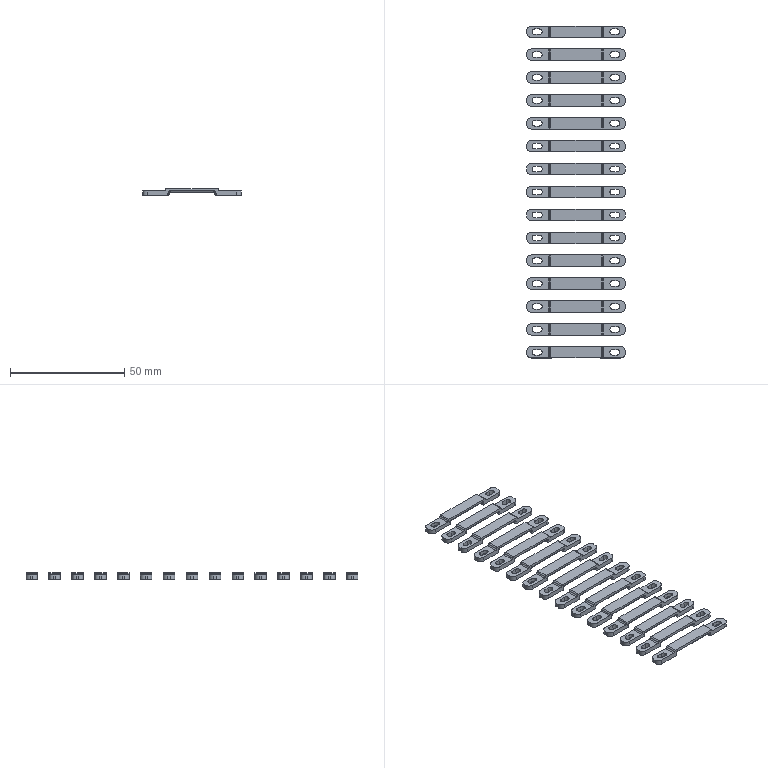NC program | NX | posted with a generic post | part box 43 x 145 x 3 mm
Lines 3017 to 4403 of 17881:
(PLANAR_MILL_COPY_COPY_COPY_COPY_COPY_COPY_1 , TOOL : D6A45)
N6014 T01 M6
N6016 G54
N6018 G17 G0 G90 X-73.9 Y-15.667 S9500 M3
N6020 G43 Z30. H1
N6022 Z0.5
N6024 G94 G1 Z-1. F1250.
N6026 G3 X-73.4 Y-14.801 R1.
N6028 G1 Y-10.5
N6030 X-73.383 Y-10.328
N6032 X-73.341 Y-10.108
N6034 G2 X-73.181 Y-9.746 R0.9
N6036 G1 X-73.065 Y-9.588
N6038 G2 X-72.775 Y-9.334 R0.9
N6040 G1 X-72.61 Y-9.243
N6042 G2 X-72.332 Y-9.145 R0.9
N6044 G1 X-72.156 Y-9.114
N6046 X-72. Y-9.1
N6048 X-68.
N6050 X-67.844 Y-9.114
N6052 X-67.668 Y-9.145
N6054 G2 X-67.39 Y-9.243 R0.9
N6056 G1 X-67.225 Y-9.334
N6058 G2 X-66.935 Y-9.588 R0.9
N6060 G1 X-66.819 Y-9.746
N6062 G2 X-66.659 Y-10.108 R0.9
N6064 G1 X-66.617 Y-10.328
N6066 X-66.6 Y-10.5
N6068 Y-19.5
N6070 G2 X-69.5 Y-22.4 R2.9
N6072 G1 X-70.5
N6074 G2 X-73.4 Y-19.5 R2.9
N6076 G1 Y-14.801
N6078 G3 X-73.9 Y-13.935 R1.
N6080 G1 Z0.5
N6082 G0 Z30.
N6084 X-70.2 Y-17.866
N6086 Z0.5
N6088 G1 Z-1.
N6090 G3 X-69.7 Y-17. R1.
N6092 G1 Y-16.
N6094 G3 X-70. Y-15.7 R0.3
N6096 X-70.3 Y-16. R0.3
N6098 G1 Y-18.
N6100 G3 X-70. Y-18.3 R0.3
N6102 X-69.7 Y-18. R0.3
N6104 G1 Y-17.
N6106 G3 X-70.2 Y-16.134 R1.
N6108 G1 Z0.5
N6110 G0 Z30.
N6112 X-60.2 Y-17.866
N6114 Z0.5
N6116 G1 Z-1.
N6118 G3 X-59.7 Y-17. R1.
N6120 G1 Y-16.
N6122 G3 X-60. Y-15.7 R0.3
N6124 X-60.3 Y-16. R0.3
N6126 G1 Y-18.
N6128 G3 X-60. Y-18.3 R0.3
N6130 X-59.7 Y-18. R0.3
N6132 G1 Y-17.
N6134 G3 X-60.2 Y-16.134 R1.
N6136 G1 Z0.5
N6138 G0 Z30.
N6140 X-56.1 Y-13.935
N6142 Z0.5
N6144 G1 Z-1.
N6146 G3 X-56.6 Y-14.801 R1.
N6148 G1 Y-19.5
N6150 G2 X-59.5 Y-22.4 R2.9
N6152 G1 X-60.5
N6154 G2 X-63.4 Y-19.5 R2.9
N6156 G1 Y-10.5
N6158 X-63.383 Y-10.328
N6160 X-63.341 Y-10.108
N6162 G2 X-63.181 Y-9.746 R0.9
N6164 G1 X-63.065 Y-9.588
N6166 G2 X-62.775 Y-9.334 R0.9
N6168 G1 X-62.61 Y-9.243
N6170 G2 X-62.332 Y-9.145 R0.9
N6172 G1 X-62.156 Y-9.114
N6174 X-62. Y-9.1
N6176 X-58.
N6178 X-57.844 Y-9.114
N6180 X-57.668 Y-9.145
N6182 G2 X-57.39 Y-9.243 R0.9
N6184 G1 X-57.225 Y-9.334
N6186 G2 X-56.935 Y-9.588 R0.9
N6188 G1 X-56.819 Y-9.746
N6190 G2 X-56.659 Y-10.108 R0.9
N6192 G1 X-56.617 Y-10.328
N6194 X-56.6 Y-10.5
N6196 Y-14.801
N6198 G3 X-56.1 Y-15.667 R1.
N6200 G1 Z0.5
N6202 G0 Z30.
N6204 X-53.9
N6206 Z0.5
N6208 G1 Z-1.
N6210 G3 X-53.4 Y-14.801 R1.
N6212 G1 Y-10.5
N6214 X-53.383 Y-10.328
N6216 X-53.341 Y-10.108
N6218 G2 X-53.181 Y-9.746 R0.9
N6220 G1 X-53.065 Y-9.588
N6222 G2 X-52.775 Y-9.334 R0.9
N6224 G1 X-52.61 Y-9.243
N6226 G2 X-52.332 Y-9.145 R0.9
N6228 G1 X-52.156 Y-9.114
N6230 X-52. Y-9.1
N6232 X-48.
N6234 X-47.844 Y-9.114
N6236 X-47.668 Y-9.145
N6238 G2 X-47.39 Y-9.243 R0.9
N6240 G1 X-47.225 Y-9.334
N6242 G2 X-46.935 Y-9.588 R0.9
N6244 G1 X-46.819 Y-9.746
N6246 G2 X-46.659 Y-10.108 R0.9
N6248 G1 X-46.617 Y-10.328
N6250 X-46.6 Y-10.5
N6252 Y-19.5
N6254 G2 X-49.5 Y-22.4 R2.9
N6256 G1 X-50.5
N6258 G2 X-53.4 Y-19.5 R2.9
N6260 G1 Y-14.801
N6262 G3 X-53.9 Y-13.935 R1.
N6264 G1 Z0.5
N6266 G0 Z30.
N6268 X-50.2 Y-17.866
N6270 Z0.5
N6272 G1 Z-1.
N6274 G3 X-49.7 Y-17. R1.
N6276 G1 Y-16.
N6278 G3 X-50. Y-15.7 R0.3
N6280 X-50.3 Y-16. R0.3
N6282 G1 Y-18.
N6284 G3 X-50. Y-18.3 R0.3
N6286 X-49.7 Y-18. R0.3
N6288 G1 Y-17.
N6290 G3 X-50.2 Y-16.134 R1.
N6292 G1 Z0.5
N6294 G0 Z30.
N6296 X-40.2 Y-17.866
N6298 Z0.5
N6300 G1 Z-1.
N6302 G3 X-39.7 Y-17. R1.
N6304 G1 Y-16.
N6306 G3 X-40. Y-15.7 R0.3
N6308 X-40.3 Y-16. R0.3
N6310 G1 Y-18.
N6312 G3 X-40. Y-18.3 R0.3
N6314 X-39.7 Y-18. R0.3
N6316 G1 Y-17.
N6318 G3 X-40.2 Y-16.134 R1.
N6320 G1 Z0.5
N6322 G0 Z30.
N6324 X-36.1 Y-13.935
N6326 Z0.5
N6328 G1 Z-1.
N6330 G3 X-36.6 Y-14.801 R1.
N6332 G1 Y-19.5
N6334 G2 X-39.5 Y-22.4 R2.9
N6336 G1 X-40.5
N6338 G2 X-43.4 Y-19.5 R2.9
N6340 G1 Y-10.5
N6342 X-43.383 Y-10.328
N6344 X-43.341 Y-10.108
N6346 G2 X-43.181 Y-9.746 R0.9
N6348 G1 X-43.065 Y-9.588
N6350 G2 X-42.775 Y-9.334 R0.9
N6352 G1 X-42.61 Y-9.243
N6354 G2 X-42.332 Y-9.145 R0.9
N6356 G1 X-42.156 Y-9.114
N6358 X-42. Y-9.1
N6360 X-38.
N6362 X-37.844 Y-9.114
N6364 X-37.668 Y-9.145
N6366 G2 X-37.39 Y-9.243 R0.9
N6368 G1 X-37.225 Y-9.334
N6370 G2 X-36.935 Y-9.588 R0.9
N6372 G1 X-36.819 Y-9.746
N6374 G2 X-36.659 Y-10.108 R0.9
N6376 G1 X-36.617 Y-10.328
N6378 X-36.6 Y-10.5
N6380 Y-14.801
N6382 G3 X-36.1 Y-15.667 R1.
N6384 G1 Z0.5
N6386 G0 Z30.
N6388 X-33.9
N6390 Z0.5
N6392 G1 Z-1.
N6394 G3 X-33.4 Y-14.801 R1.
N6396 G1 Y-10.5
N6398 X-33.383 Y-10.328
N6400 X-33.341 Y-10.108
N6402 G2 X-33.181 Y-9.746 R0.9
N6404 G1 X-33.065 Y-9.588
N6406 G2 X-32.775 Y-9.334 R0.9
N6408 G1 X-32.61 Y-9.243
N6410 G2 X-32.332 Y-9.145 R0.9
N6412 G1 X-32.156 Y-9.114
N6414 X-32. Y-9.1
N6416 X-28.
N6418 X-27.844 Y-9.114
N6420 X-27.668 Y-9.145
N6422 G2 X-27.39 Y-9.243 R0.9
N6424 G1 X-27.225 Y-9.334
N6426 G2 X-26.935 Y-9.588 R0.9
N6428 G1 X-26.819 Y-9.746
N6430 G2 X-26.659 Y-10.108 R0.9
N6432 G1 X-26.617 Y-10.328
N6434 X-26.6 Y-10.5
N6436 Y-19.5
N6438 G2 X-29.5 Y-22.4 R2.9
N6440 G1 X-30.5
N6442 G2 X-33.4 Y-19.5 R2.9
N6444 G1 Y-14.801
N6446 G3 X-33.9 Y-13.935 R1.
N6448 G1 Z0.5
N6450 G0 Z30.
N6452 X-30.2 Y-17.866
N6454 Z0.5
N6456 G1 Z-1.
N6458 G3 X-29.7 Y-17. R1.
N6460 G1 Y-16.
N6462 G3 X-30. Y-15.7 R0.3
N6464 X-30.3 Y-16. R0.3
N6466 G1 Y-18.
N6468 G3 X-30. Y-18.3 R0.3
N6470 X-29.7 Y-18. R0.3
N6472 G1 Y-17.
N6474 G3 X-30.2 Y-16.134 R1.
N6476 G1 Z0.5
N6478 G0 Z30.
N6480 X-23.9 Y-15.667
N6482 Z0.5
N6484 G1 Z-1.
N6486 G3 X-23.4 Y-14.801 R1.
N6488 G1 Y-10.5
N6490 X-23.383 Y-10.328
N6492 X-23.341 Y-10.108
N6494 G2 X-23.181 Y-9.746 R0.9
N6496 G1 X-23.065 Y-9.588
N6498 G2 X-22.775 Y-9.334 R0.9
N6500 G1 X-22.61 Y-9.243
N6502 G2 X-22.332 Y-9.145 R0.9
N6504 G1 X-22.156 Y-9.114
N6506 X-22. Y-9.1
N6508 X-18.
N6510 X-17.844 Y-9.114
N6512 X-17.668 Y-9.145
N6514 G2 X-17.39 Y-9.243 R0.9
N6516 G1 X-17.225 Y-9.334
N6518 G2 X-16.935 Y-9.588 R0.9
N6520 G1 X-16.819 Y-9.746
N6522 G2 X-16.659 Y-10.108 R0.9
N6524 G1 X-16.617 Y-10.328
N6526 X-16.6 Y-10.5
N6528 Y-19.5
N6530 G2 X-19.5 Y-22.4 R2.9
N6532 G1 X-20.5
N6534 G2 X-23.4 Y-19.5 R2.9
N6536 G1 Y-14.801
N6538 G3 X-23.9 Y-13.935 R1.
N6540 G1 Z0.5
N6542 G0 Z30.
N6544 X-20.2 Y-17.866
N6546 Z0.5
N6548 G1 Z-1.
N6550 G3 X-19.7 Y-17. R1.
N6552 G1 Y-16.
N6554 G3 X-20. Y-15.7 R0.3
N6556 X-20.3 Y-16. R0.3
N6558 G1 Y-18.
N6560 G3 X-20. Y-18.3 R0.3
N6562 X-19.7 Y-18. R0.3
N6564 G1 Y-17.
N6566 G3 X-20.2 Y-16.134 R1.
N6568 G1 Z0.5
N6570 G0 Z30.
N6572 X-10.2 Y-17.866
N6574 Z0.5
N6576 G1 Z-1.
N6578 G3 X-9.7 Y-17. R1.
N6580 G1 Y-16.
N6582 G3 X-10. Y-15.7 R0.3
N6584 X-10.3 Y-16. R0.3
N6586 G1 Y-18.
N6588 G3 X-10. Y-18.3 R0.3
N6590 X-9.7 Y-18. R0.3
N6592 G1 Y-17.
N6594 G3 X-10.2 Y-16.134 R1.
N6596 G1 Z0.5
N6598 G0 Z30.
N6600 X-6.1 Y-13.935
N6602 Z0.5
N6604 G1 Z-1.
N6606 G3 X-6.6 Y-14.801 R1.
N6608 G1 Y-19.5
N6610 G2 X-9.5 Y-22.4 R2.9
N6612 G1 X-10.5
N6614 G2 X-13.4 Y-19.5 R2.9
N6616 G1 Y-10.5
N6618 X-13.383 Y-10.328
N6620 X-13.341 Y-10.108
N6622 G2 X-13.181 Y-9.746 R0.9
N6624 G1 X-13.065 Y-9.588
N6626 G2 X-12.775 Y-9.334 R0.9
N6628 G1 X-12.61 Y-9.243
N6630 G2 X-12.332 Y-9.145 R0.9
N6632 G1 X-12.156 Y-9.114
N6634 X-12. Y-9.1
N6636 X-8.
N6638 X-7.844 Y-9.114
N6640 X-7.668 Y-9.145
N6642 G2 X-7.39 Y-9.243 R0.9
N6644 G1 X-7.225 Y-9.334
N6646 G2 X-6.935 Y-9.588 R0.9
N6648 G1 X-6.819 Y-9.746
N6650 G2 X-6.659 Y-10.108 R0.9
N6652 G1 X-6.617 Y-10.328
N6654 X-6.6 Y-10.5
N6656 Y-14.801
N6658 G3 X-6.1 Y-15.667 R1.
N6660 G1 Z0.5
N6662 G0 Z30.
N6664 X-3.9
N6666 Z0.5
N6668 G1 Z-1.
N6670 G3 X-3.4 Y-14.801 R1.
N6672 G1 Y-10.5
N6674 X-3.383 Y-10.328
N6676 X-3.341 Y-10.108
N6678 G2 X-3.181 Y-9.746 R0.9
N6680 G1 X-3.065 Y-9.588
N6682 G2 X-2.775 Y-9.334 R0.9
N6684 G1 X-2.61 Y-9.243
N6686 G2 X-2.332 Y-9.145 R0.9
N6688 G1 X-2.156 Y-9.114
N6690 X-2. Y-9.1
N6692 X2.
N6694 X2.156 Y-9.114
N6696 X2.332 Y-9.145
N6698 G2 X2.61 Y-9.243 R0.9
N6700 G1 X2.775 Y-9.334
N6702 G2 X3.065 Y-9.588 R0.9
N6704 G1 X3.181 Y-9.746
N6706 G2 X3.341 Y-10.108 R0.9
N6708 G1 X3.383 Y-10.328
N6710 X3.4 Y-10.5
N6712 Y-19.5
N6714 G2 X0.5 Y-22.4 R2.9
N6716 G1 X-0.5
N6718 G2 X-3.4 Y-19.5 R2.9
N6720 G1 Y-14.801
N6722 G3 X-3.9 Y-13.935 R1.
N6724 G1 Z0.5
N6726 G0 Z30.
N6728 X-0.2 Y-17.866
N6730 Z0.5
N6732 G1 Z-1.
N6734 G3 X0.3 Y-17. R1.
N6736 G1 Y-16.
N6738 G3 X0. Y-15.7 R0.3
N6740 X-0.3 Y-16. R0.3
N6742 G1 Y-18.
N6744 G3 X0. Y-18.3 R0.3
N6746 X0.3 Y-18. R0.3
N6748 G1 Y-17.
N6750 G3 X-0.2 Y-16.134 R1.
N6752 G1 Z0.5
N6754 G0 Z30.
N6756 X9.8 Y-17.866
N6758 Z0.5
N6760 G1 Z-1.
N6762 G3 X10.3 Y-17. R1.
N6764 G1 Y-16.
N6766 G3 X10. Y-15.7 R0.3
N6768 X9.7 Y-16. R0.3
N6770 G1 Y-18.
N6772 G3 X10. Y-18.3 R0.3
N6774 X10.3 Y-18. R0.3
N6776 G1 Y-17.
N6778 G3 X9.8 Y-16.134 R1.
N6780 G1 Z0.5
N6782 G0 Z30.
N6784 X13.9 Y-13.935
N6786 Z0.5
N6788 G1 Z-1.
N6790 G3 X13.4 Y-14.801 R1.
N6792 G1 Y-19.5
N6794 G2 X10.5 Y-22.4 R2.9
N6796 G1 X9.5
N6798 G2 X6.6 Y-19.5 R2.9
N6800 G1 Y-10.5
N6802 X6.617 Y-10.328
N6804 X6.659 Y-10.108
N6806 G2 X6.819 Y-9.746 R0.9
N6808 G1 X6.935 Y-9.588
N6810 G2 X7.225 Y-9.334 R0.9
N6812 G1 X7.39 Y-9.243
N6814 G2 X7.668 Y-9.145 R0.9
N6816 G1 X7.844 Y-9.114
N6818 X8. Y-9.1
N6820 X12.
N6822 X12.156 Y-9.114
N6824 X12.332 Y-9.145
N6826 G2 X12.61 Y-9.243 R0.9
N6828 G1 X12.775 Y-9.334
N6830 G2 X13.065 Y-9.588 R0.9
N6832 G1 X13.181 Y-9.746
N6834 G2 X13.341 Y-10.108 R0.9
N6836 G1 X13.383 Y-10.328
N6838 X13.4 Y-10.5
N6840 Y-14.801
N6842 G3 X13.9 Y-15.667 R1.
N6844 G1 Z0.5
N6846 G0 Z30.
N6848 X16.1
N6850 Z0.5
N6852 G1 Z-1.
N6854 G3 X16.6 Y-14.801 R1.
N6856 G1 Y-10.5
N6858 X16.617 Y-10.328
N6860 X16.659 Y-10.108
N6862 G2 X16.819 Y-9.746 R0.9
N6864 G1 X16.935 Y-9.588
N6866 G2 X17.225 Y-9.334 R0.9
N6868 G1 X17.39 Y-9.243
N6870 G2 X17.668 Y-9.145 R0.9
N6872 G1 X17.844 Y-9.114
N6874 X18. Y-9.1
N6876 X22.
N6878 X22.156 Y-9.114
N6880 X22.332 Y-9.145
N6882 G2 X22.61 Y-9.243 R0.9
N6884 G1 X22.775 Y-9.334
N6886 G2 X23.065 Y-9.588 R0.9
N6888 G1 X23.181 Y-9.746
N6890 G2 X23.341 Y-10.108 R0.9
N6892 G1 X23.383 Y-10.328
N6894 X23.4 Y-10.5
N6896 Y-19.5
N6898 G2 X20.5 Y-22.4 R2.9
N6900 G1 X19.5
N6902 G2 X16.6 Y-19.5 R2.9
N6904 G1 Y-14.801
N6906 G3 X16.1 Y-13.935 R1.
N6908 G1 Z0.5
N6910 G0 Z30.
N6912 X19.8 Y-17.866
N6914 Z0.5
N6916 G1 Z-1.
N6918 G3 X20.3 Y-17. R1.
N6920 G1 Y-16.
N6922 G3 X20. Y-15.7 R0.3
N6924 X19.7 Y-16. R0.3
N6926 G1 Y-18.
N6928 G3 X20. Y-18.3 R0.3
N6930 X20.3 Y-18. R0.3
N6932 G1 Y-17.
N6934 G3 X19.8 Y-16.134 R1.
N6936 G1 Z0.5
N6938 G0 Z30.
N6940 X29.8 Y-17.866
N6942 Z0.5
N6944 G1 Z-1.
N6946 G3 X30.3 Y-17. R1.
N6948 G1 Y-16.
N6950 G3 X30. Y-15.7 R0.3
N6952 X29.7 Y-16. R0.3
N6954 G1 Y-18.
N6956 G3 X30. Y-18.3 R0.3
N6958 X30.3 Y-18. R0.3
N6960 G1 Y-17.
N6962 G3 X29.8 Y-16.134 R1.
N6964 G1 Z0.5
N6966 G0 Z30.
N6968 X26.1 Y-15.667
N6970 Z0.5
N6972 G1 Z-1.
N6974 G3 X26.6 Y-14.801 R1.
N6976 G1 Y-10.5
N6978 X26.617 Y-10.328
N6980 X26.659 Y-10.108
N6982 G2 X26.819 Y-9.746 R0.9
N6984 G1 X26.935 Y-9.588
N6986 G2 X27.225 Y-9.334 R0.9
N6988 G1 X27.39 Y-9.243
N6990 G2 X27.668 Y-9.145 R0.9
N6992 G1 X27.844 Y-9.114
N6994 X28. Y-9.1
N6996 X32.
N6998 X32.156 Y-9.114
N7000 X32.332 Y-9.145
N7002 G2 X32.61 Y-9.243 R0.9
N7004 G1 X32.775 Y-9.334
N7006 G2 X33.065 Y-9.588 R0.9
N7008 G1 X33.181 Y-9.746
N7010 G2 X33.341 Y-10.108 R0.9
N7012 G1 X33.383 Y-10.328
N7014 X33.4 Y-10.5
N7016 Y-19.5
N7018 G2 X30.5 Y-22.4 R2.9
N7020 G1 X29.5
N7022 G2 X26.6 Y-19.5 R2.9
N7024 G1 Y-14.801
N7026 G3 X26.1 Y-13.935 R1.
N7028 G1 Z0.5
N7030 G0 Z30.
N7032 X36.1 Y-15.667
N7034 Z0.5
N7036 G1 Z-1.
N7038 G3 X36.6 Y-14.801 R1.
N7040 G1 Y-10.5
N7042 X36.617 Y-10.328
N7044 X36.659 Y-10.108
N7046 G2 X36.819 Y-9.746 R0.9
N7048 G1 X36.935 Y-9.588
N7050 G2 X37.225 Y-9.334 R0.9
N7052 G1 X37.39 Y-9.243
N7054 G2 X37.668 Y-9.145 R0.9
N7056 G1 X37.844 Y-9.114
N7058 X38. Y-9.1
N7060 X42.
N7062 X42.156 Y-9.114
N7064 X42.332 Y-9.145
N7066 G2 X42.61 Y-9.243 R0.9
N7068 G1 X42.775 Y-9.334
N7070 G2 X43.065 Y-9.588 R0.9
N7072 G1 X43.181 Y-9.746
N7074 G2 X43.341 Y-10.108 R0.9
N7076 G1 X43.383 Y-10.328
N7078 X43.4 Y-10.5
N7080 Y-19.5
N7082 G2 X40.5 Y-22.4 R2.9
N7084 G1 X39.5
N7086 G2 X36.6 Y-19.5 R2.9
N7088 G1 Y-14.801
N7090 G3 X36.1 Y-13.935 R1.
N7092 G1 Z0.5
N7094 G0 Z30.
N7096 X39.8 Y-17.866
N7098 Z0.5
N7100 G1 Z-1.
N7102 G3 X40.3 Y-17. R1.
N7104 G1 Y-16.
N7106 G3 X40. Y-15.7 R0.3
N7108 X39.7 Y-16. R0.3
N7110 G1 Y-18.
N7112 G3 X40. Y-18.3 R0.3
N7114 X40.3 Y-18. R0.3
N7116 G1 Y-17.
N7118 G3 X39.8 Y-16.134 R1.
N7120 G1 Z0.5
N7122 G0 Z30.
N7124 X49.8 Y-17.866
N7126 Z0.5
N7128 G1 Z-1.
N7130 G3 X50.3 Y-17. R1.
N7132 G1 Y-16.
N7134 G3 X50. Y-15.7 R0.3
N7136 X49.7 Y-16. R0.3
N7138 G1 Y-18.
N7140 G3 X50. Y-18.3 R0.3
N7142 X50.3 Y-18. R0.3
N7144 G1 Y-17.
N7146 G3 X49.8 Y-16.134 R1.
N7148 G1 Z0.5
N7150 G0 Z30.
N7152 X46.1 Y-15.667
N7154 Z0.5
N7156 G1 Z-1.
N7158 G3 X46.6 Y-14.801 R1.
N7160 G1 Y-10.5
N7162 X46.617 Y-10.328
N7164 X46.659 Y-10.108
N7166 G2 X46.819 Y-9.746 R0.9
N7168 G1 X46.935 Y-9.588
N7170 G2 X47.225 Y-9.334 R0.9
N7172 G1 X47.39 Y-9.243
N7174 G2 X47.668 Y-9.145 R0.9
N7176 G1 X47.844 Y-9.114
N7178 X48. Y-9.1
N7180 X52.
N7182 X52.156 Y-9.114
N7184 X52.332 Y-9.145
N7186 G2 X52.61 Y-9.243 R0.9
N7188 G1 X52.775 Y-9.334
N7190 G2 X53.065 Y-9.588 R0.9
N7192 G1 X53.181 Y-9.746
N7194 G2 X53.341 Y-10.108 R0.9
N7196 G1 X53.383 Y-10.328
N7198 X53.4 Y-10.5
N7200 Y-19.5
N7202 G2 X50.5 Y-22.4 R2.9
N7204 G1 X49.5
N7206 G2 X46.6 Y-19.5 R2.9
N7208 G1 Y-14.801
N7210 G3 X46.1 Y-13.935 R1.
N7212 G1 Z0.5
N7214 G0 Z30.
N7216 X56.1 Y-15.667
N7218 Z0.5
N7220 G1 Z-1.
N7222 G3 X56.6 Y-14.801 R1.
N7224 G1 Y-10.5
N7226 X56.617 Y-10.328
N7228 X56.659 Y-10.108
N7230 G2 X56.819 Y-9.746 R0.9
N7232 G1 X56.935 Y-9.588
N7234 G2 X57.225 Y-9.334 R0.9
N7236 G1 X57.39 Y-9.243
N7238 G2 X57.668 Y-9.145 R0.9
N7240 G1 X57.844 Y-9.114
N7242 X58. Y-9.1
N7244 X62.
N7246 X62.156 Y-9.114
N7248 X62.332 Y-9.145
N7250 G2 X62.61 Y-9.243 R0.9
N7252 G1 X62.775 Y-9.334
N7254 G2 X63.065 Y-9.588 R0.9
N7256 G1 X63.181 Y-9.746
N7258 G2 X63.341 Y-10.108 R0.9
N7260 G1 X63.383 Y-10.328
N7262 X63.4 Y-10.5
N7264 Y-19.5
N7266 G2 X60.5 Y-22.4 R2.9
N7268 G1 X59.5
N7270 G2 X56.6 Y-19.5 R2.9
N7272 G1 Y-14.801
N7274 G3 X56.1 Y-13.935 R1.
N7276 G1 Z0.5
N7278 G0 Z30.
N7280 X59.8 Y-17.866
N7282 Z0.5
N7284 G1 Z-1.
N7286 G3 X60.3 Y-17. R1.
N7288 G1 Y-16.
N7290 G3 X60. Y-15.7 R0.3
N7292 X59.7 Y-16. R0.3
N7294 G1 Y-18.
N7296 G3 X60. Y-18.3 R0.3
N7298 X60.3 Y-18. R0.3
N7300 G1 Y-17.
N7302 G3 X59.8 Y-16.134 R1.
N7304 G1 Z0.5
N7306 G0 Z30.
N7308 X69.8 Y-17.866
N7310 Z0.5
N7312 G1 Z-1.
N7314 G3 X70.3 Y-17. R1.
N7316 G1 Y-16.
N7318 G3 X70. Y-15.7 R0.3
N7320 X69.7 Y-16. R0.3
N7322 G1 Y-18.
N7324 G3 X70. Y-18.3 R0.3
N7326 X70.3 Y-18. R0.3
N7328 G1 Y-17.
N7330 G3 X69.8 Y-16.134 R1.
N7332 G1 Z0.5
N7334 G0 Z30.
N7336 X73.9 Y-13.935
N7338 Z0.5
N7340 G1 Z-1.
N7342 G3 X73.4 Y-14.801 R1.
N7344 G1 Y-19.5
N7346 G2 X70.5 Y-22.4 R2.9
N7348 G1 X69.5
N7350 G2 X66.6 Y-19.5 R2.9
N7352 G1 Y-10.5
N7354 X66.617 Y-10.328
N7356 X66.659 Y-10.108
N7358 G2 X66.819 Y-9.746 R0.9
N7360 G1 X66.935 Y-9.588
N7362 G2 X67.225 Y-9.334 R0.9
N7364 G1 X67.39 Y-9.243
N7366 G2 X67.668 Y-9.145 R0.9
N7368 G1 X67.844 Y-9.114
N7370 X68. Y-9.1
N7372 X72.
N7374 X72.156 Y-9.114
N7376 X72.332 Y-9.145
N7378 G2 X72.61 Y-9.243 R0.9
N7380 G1 X72.775 Y-9.334
N7382 G2 X73.065 Y-9.588 R0.9
N7384 G1 X73.181 Y-9.746
N7386 G2 X73.341 Y-10.108 R0.9
N7388 G1 X73.383 Y-10.328
N7390 X73.4 Y-10.5
N7392 Y-14.801
N7394 G3 X73.9 Y-15.667 R1.
N7396 G1 Z0.5
N7398 G0 Z30.
N7400 Y15.667
N7402 Z0.5
N7404 G1 Z-1.
N7406 G3 X73.4 Y14.801 R1.
N7408 G1 Y10.5
N7410 X73.383 Y10.328
N7412 X73.341 Y10.108
N7414 G2 X73.181 Y9.746 R0.9
N7416 G1 X73.065 Y9.588
N7418 G2 X72.775 Y9.334 R0.9
N7420 G1 X72.61 Y9.243
N7422 G2 X72.332 Y9.145 R0.9
N7424 G1 X72.156 Y9.114
N7426 X72. Y9.1
N7428 X68.
N7430 X67.844 Y9.114
N7432 X67.668 Y9.145
N7434 G2 X67.39 Y9.243 R0.9
N7436 G1 X67.225 Y9.334
N7438 G2 X66.935 Y9.588 R0.9
N7440 G1 X66.819 Y9.746
N7442 G2 X66.659 Y10.108 R0.9
N7444 G1 X66.617 Y10.328
N7446 X66.6 Y10.5
N7448 Y19.5
N7450 G2 X69.5 Y22.4 R2.9
N7452 G1 X70.5
N7454 G2 X73.4 Y19.5 R2.9
N7456 G1 Y14.801
N7458 G3 X73.9 Y13.935 R1.
N7460 G1 Z0.5
N7462 G0 Z30.
N7464 X69.8 Y16.134
N7466 Z0.5
N7468 G1 Z-1.
N7470 G3 X70.3 Y17. R1.
N7472 G1 Y18.
N7474 G3 X70. Y18.3 R0.3
N7476 X69.7 Y18. R0.3
N7478 G1 Y16.
N7480 G3 X70. Y15.7 R0.3
N7482 X70.3 Y16. R0.3
N7484 G1 Y17.
N7486 G3 X69.8 Y17.866 R1.
N7488 G1 Z0.5
N7490 G0 Z30.
N7492 X59.8 Y16.134
N7494 Z0.5
N7496 G1 Z-1.
N7498 G3 X60.3 Y17. R1.
N7500 G1 Y18.
N7502 G3 X60. Y18.3 R0.3
N7504 X59.7 Y18. R0.3
N7506 G1 Y16.
N7508 G3 X60. Y15.7 R0.3
N7510 X60.3 Y16. R0.3
N7512 G1 Y17.
N7514 G3 X59.8 Y17.866 R1.
N7516 G1 Z0.5
N7518 G0 Z30.
N7520 X63.9 Y15.667
N7522 Z0.5
N7524 G1 Z-1.
N7526 G3 X63.4 Y14.801 R1.
N7528 G1 Y10.5
N7530 X63.383 Y10.328
N7532 X63.341 Y10.108
N7534 G2 X63.181 Y9.746 R0.9
N7536 G1 X63.065 Y9.588
N7538 G2 X62.775 Y9.334 R0.9
N7540 G1 X62.61 Y9.243
N7542 G2 X62.332 Y9.145 R0.9
N7544 G1 X62.156 Y9.114
N7546 X62. Y9.1
N7548 X58.
N7550 X57.844 Y9.114
N7552 X57.668 Y9.145
N7554 G2 X57.39 Y9.243 R0.9
N7556 G1 X57.225 Y9.334
N7558 G2 X56.935 Y9.588 R0.9
N7560 G1 X56.819 Y9.746
N7562 G2 X56.659 Y10.108 R0.9
N7564 G1 X56.617 Y10.328
N7566 X56.6 Y10.5
N7568 Y19.5
N7570 G2 X59.5 Y22.4 R2.9
N7572 G1 X60.5
N7574 G2 X63.4 Y19.5 R2.9
N7576 G1 Y14.801
N7578 G3 X63.9 Y13.935 R1.
N7580 G1 Z0.5
N7582 G0 Z30.
N7584 X53.9 Y15.667
N7586 Z0.5
N7588 G1 Z-1.
N7590 G3 X53.4 Y14.801 R1.
N7592 G1 Y10.5
N7594 X53.383 Y10.328
N7596 X53.341 Y10.108
N7598 G2 X53.181 Y9.746 R0.9
N7600 G1 X53.065 Y9.588
N7602 G2 X52.775 Y9.334 R0.9
N7604 G1 X52.61 Y9.243
N7606 G2 X52.332 Y9.145 R0.9
N7608 G1 X52.156 Y9.114
N7610 X52. Y9.1
N7612 X48.
N7614 X47.844 Y9.114
N7616 X47.668 Y9.145
N7618 G2 X47.39 Y9.243 R0.9
N7620 G1 X47.225 Y9.334
N7622 G2 X46.935 Y9.588 R0.9
N7624 G1 X46.819 Y9.746
N7626 G2 X46.659 Y10.108 R0.9
N7628 G1 X46.617 Y10.328
N7630 X46.6 Y10.5
N7632 Y19.5
N7634 G2 X49.5 Y22.4 R2.9
N7636 G1 X50.5
N7638 G2 X53.4 Y19.5 R2.9
N7640 G1 Y14.801
N7642 G3 X53.9 Y13.935 R1.
N7644 G1 Z0.5
N7646 G0 Z30.
N7648 X50.2 Y17.866
N7650 Z0.5
N7652 G1 Z-1.
N7654 G3 X49.7 Y17. R1.
N7656 G1 Y16.
N7658 G3 X50. Y15.7 R0.3
N7660 X50.3 Y16. R0.3
N7662 G1 Y18.
N7664 G3 X50. Y18.3 R0.3
N7666 X49.7 Y18. R0.3
N7668 G1 Y17.
N7670 G3 X50.2 Y16.134 R1.
N7672 G1 Z0.5
N7674 G0 Z30.
N7676 X39.8
N7678 Z0.5
N7680 G1 Z-1.
N7682 G3 X40.3 Y17. R1.
N7684 G1 Y18.
N7686 G3 X40. Y18.3 R0.3
N7688 X39.7 Y18. R0.3
N7690 G1 Y16.
N7692 G3 X40. Y15.7 R0.3
N7694 X40.3 Y16. R0.3
N7696 G1 Y17.
N7698 G3 X39.8 Y17.866 R1.
N7700 G1 Z0.5
N7702 G0 Z30.
N7704 X43.9 Y15.667
N7706 Z0.5
N7708 G1 Z-1.
N7710 G3 X43.4 Y14.801 R1.
N7712 G1 Y10.5
N7714 X43.383 Y10.328
N7716 X43.341 Y10.108
N7718 G2 X43.181 Y9.746 R0.9
N7720 G1 X43.065 Y9.588
N7722 G2 X42.775 Y9.334 R0.9
N7724 G1 X42.61 Y9.243
N7726 G2 X42.332 Y9.145 R0.9
N7728 G1 X42.156 Y9.114
N7730 X42. Y9.1
N7732 X38.
N7734 X37.844 Y9.114
N7736 X37.668 Y9.145
N7738 G2 X37.39 Y9.243 R0.9
N7740 G1 X37.225 Y9.334
N7742 G2 X36.935 Y9.588 R0.9
N7744 G1 X36.819 Y9.746
N7746 G2 X36.659 Y10.108 R0.9
N7748 G1 X36.617 Y10.328
N7750 X36.6 Y10.5
N7752 Y19.5
N7754 G2 X39.5 Y22.4 R2.9
N7756 G1 X40.5
N7758 G2 X43.4 Y19.5 R2.9
N7760 G1 Y14.801
N7762 G3 X43.9 Y13.935 R1.
N7764 G1 Z0.5
N7766 G0 Z30.
N7768 X33.9 Y15.667
N7770 Z0.5
N7772 G1 Z-1.
N7774 G3 X33.4 Y14.801 R1.
N7776 G1 Y10.5
N7778 X33.383 Y10.328
N7780 X33.341 Y10.108
N7782 G2 X33.181 Y9.746 R0.9
N7784 G1 X33.065 Y9.588
N7786 G2 X32.775 Y9.334 R0.9
N7788 G1 X32.61 Y9.243
N7790 G2 X32.332 Y9.145 R0.9
N7792 G1 X32.156 Y9.114
N7794 X32. Y9.1
N7796 X28.
N7798 X27.844 Y9.114
N7800 X27.668 Y9.145
N7802 G2 X27.39 Y9.243 R0.9
N7804 G1 X27.225 Y9.334
N7806 G2 X26.935 Y9.588 R0.9
N7808 G1 X26.819 Y9.746
N7810 G2 X26.659 Y10.108 R0.9
N7812 G1 X26.617 Y10.328
N7814 X26.6 Y10.5
N7816 Y19.5
N7818 G2 X29.5 Y22.4 R2.9
N7820 G1 X30.5
N7822 G2 X33.4 Y19.5 R2.9
N7824 G1 Y14.801
N7826 G3 X33.9 Y13.935 R1.
N7828 G1 Z0.5
N7830 G0 Z30.
N7832 X29.8 Y16.134
N7834 Z0.5
N7836 G1 Z-1.
N7838 G3 X30.3 Y17. R1.
N7840 G1 Y18.
N7842 G3 X30. Y18.3 R0.3
N7844 X29.7 Y18. R0.3
N7846 G1 Y16.
N7848 G3 X30. Y15.7 R0.3
N7850 X30.3 Y16. R0.3
N7852 G1 Y17.
N7854 G3 X29.8 Y17.866 R1.
N7856 G1 Z0.5
N7858 G0 Z30.
N7860 X20.2
N7862 Z0.5
N7864 G1 Z-1.
N7866 G3 X19.7 Y17. R1.
N7868 G1 Y16.
N7870 G3 X20. Y15.7 R0.3
N7872 X20.3 Y16. R0.3
N7874 G1 Y18.
N7876 G3 X20. Y18.3 R0.3
N7878 X19.7 Y18. R0.3
N7880 G1 Y17.
N7882 G3 X20.2 Y16.134 R1.
N7884 G1 Z0.5
N7886 G0 Z30.
N7888 X23.9 Y15.667
N7890 Z0.5
N7892 G1 Z-1.
N7894 G3 X23.4 Y14.801 R1.
N7896 G1 Y10.5
N7898 X23.383 Y10.328
N7900 X23.341 Y10.108
N7902 G2 X23.181 Y9.746 R0.9
N7904 G1 X23.065 Y9.588
N7906 G2 X22.775 Y9.334 R0.9
N7908 G1 X22.61 Y9.243
N7910 G2 X22.332 Y9.145 R0.9
N7912 G1 X22.156 Y9.114
N7914 X22. Y9.1
N7916 X18.
N7918 X17.844 Y9.114
N7920 X17.668 Y9.145
N7922 G2 X17.39 Y9.243 R0.9
N7924 G1 X17.225 Y9.334
N7926 G2 X16.935 Y9.588 R0.9
N7928 G1 X16.819 Y9.746
N7930 G2 X16.659 Y10.108 R0.9
N7932 G1 X16.617 Y10.328
N7934 X16.6 Y10.5
N7936 Y19.5
N7938 G2 X19.5 Y22.4 R2.9
N7940 G1 X20.5
N7942 G2 X23.4 Y19.5 R2.9
N7944 G1 Y14.801
N7946 G3 X23.9 Y13.935 R1.
N7948 G1 Z0.5
N7950 G0 Z30.
N7952 X13.9 Y15.667
N7954 Z0.5
N7956 G1 Z-1.
N7958 G3 X13.4 Y14.801 R1.
N7960 G1 Y10.5
N7962 X13.383 Y10.328
N7964 X13.341 Y10.108
N7966 G2 X13.181 Y9.746 R0.9
N7968 G1 X13.065 Y9.588
N7970 G2 X12.775 Y9.334 R0.9
N7972 G1 X12.61 Y9.243
N7974 G2 X12.332 Y9.145 R0.9
N7976 G1 X12.156 Y9.114
N7978 X12. Y9.1
N7980 X8.
N7982 X7.844 Y9.114
N7984 X7.668 Y9.145
N7986 G2 X7.39 Y9.243 R0.9
N7988 G1 X7.225 Y9.334
N7990 G2 X6.935 Y9.588 R0.9
N7992 G1 X6.819 Y9.746
N7994 G2 X6.659 Y10.108 R0.9
N7996 G1 X6.617 Y10.328
N7998 X6.6 Y10.5
N8000 Y19.5
N8002 G2 X9.5 Y22.4 R2.9
N8004 G1 X10.5
N8006 G2 X13.4 Y19.5 R2.9
N8008 G1 Y14.801
N8010 G3 X13.9 Y13.935 R1.
N8012 G1 Z0.5
N8014 G0 Z30.
N8016 X9.8 Y16.134
N8018 Z0.5
N8020 G1 Z-1.
N8022 G3 X10.3 Y17. R1.
N8024 G1 Y18.
N8026 G3 X10. Y18.3 R0.3
N8028 X9.7 Y18. R0.3
N8030 G1 Y16.
N8032 G3 X10. Y15.7 R0.3
N8034 X10.3 Y16. R0.3
N8036 G1 Y17.
N8038 G3 X9.8 Y17.866 R1.
N8040 G1 Z0.5
N8042 G0 Z30.
N8044 X-0.2 Y16.134
N8046 Z0.5
N8048 G1 Z-1.
N8050 G3 X0.3 Y17. R1.
N8052 G1 Y18.
N8054 G3 X0. Y18.3 R0.3
N8056 X-0.3 Y18. R0.3
N8058 G1 Y16.
N8060 G3 X0. Y15.7 R0.3
N8062 X0.3 Y16. R0.3
N8064 G1 Y17.
N8066 G3 X-0.2 Y17.866 R1.
N8068 G1 Z0.5
N8070 G0 Z30.
N8072 X3.9 Y15.667
N8074 Z0.5
N8076 G1 Z-1.
N8078 G3 X3.4 Y14.801 R1.
N8080 G1 Y10.5
N8082 X3.383 Y10.328
N8084 X3.341 Y10.108
N8086 G2 X3.181 Y9.746 R0.9
N8088 G1 X3.065 Y9.588
N8090 G2 X2.775 Y9.334 R0.9
N8092 G1 X2.61 Y9.243
N8094 G2 X2.332 Y9.145 R0.9
N8096 G1 X2.156 Y9.114
N8098 X2. Y9.1
N8100 X-2.
N8102 X-2.156 Y9.114
N8104 X-2.332 Y9.145
N8106 G2 X-2.61 Y9.243 R0.9
N8108 G1 X-2.775 Y9.334
N8110 G2 X-3.065 Y9.588 R0.9
N8112 G1 X-3.181 Y9.746
N8114 G2 X-3.341 Y10.108 R0.9
N8116 G1 X-3.383 Y10.328
N8118 X-3.4 Y10.5
N8120 Y19.5
N8122 G2 X-0.5 Y22.4 R2.9
N8124 G1 X0.5
N8126 G2 X3.4 Y19.5 R2.9
N8128 G1 Y14.801
N8130 G3 X3.9 Y13.935 R1.
N8132 G1 Z0.5
N8134 G0 Z30.
N8136 X-6.1 Y15.667
N8138 Z0.5
N8140 G1 Z-1.
N8142 G3 X-6.6 Y14.801 R1.
N8144 G1 Y10.5
N8146 X-6.617 Y10.328
N8148 X-6.659 Y10.108
N8150 G2 X-6.819 Y9.746 R0.9
N8152 G1 X-6.935 Y9.588
N8154 G2 X-7.225 Y9.334 R0.9
N8156 G1 X-7.39 Y9.243
N8158 G2 X-7.668 Y9.145 R0.9
N8160 G1 X-7.844 Y9.114
N8162 X-8. Y9.1
N8164 X-12.
N8166 X-12.156 Y9.114
N8168 X-12.332 Y9.145
N8170 G2 X-12.61 Y9.243 R0.9
N8172 G1 X-12.775 Y9.334
N8174 G2 X-13.065 Y9.588 R0.9
N8176 G1 X-13.181 Y9.746
N8178 G2 X-13.341 Y10.108 R0.9
N8180 G1 X-13.383 Y10.328
N8182 X-13.4 Y10.5
N8184 Y19.5
N8186 G2 X-10.5 Y22.4 R2.9
N8188 G1 X-9.5
N8190 G2 X-6.6 Y19.5 R2.9
N8192 G1 Y14.801
N8194 G3 X-6.1 Y13.935 R1.
N8196 G1 Z0.5
N8198 G0 Z30.
N8200 X-9.8 Y17.866
N8202 Z0.5
N8204 G1 Z-1.
N8206 G3 X-10.3 Y17. R1.
N8208 G1 Y16.
N8210 G3 X-10. Y15.7 R0.3
N8212 X-9.7 Y16. R0.3
N8214 G1 Y18.
N8216 G3 X-10. Y18.3 R0.3
N8218 X-10.3 Y18. R0.3
N8220 G1 Y17.
N8222 G3 X-9.8 Y16.134 R1.
N8224 G1 Z0.5
N8226 G0 Z30.
N8228 X-20.2
N8230 Z0.5
N8232 G1 Z-1.
N8234 G3 X-19.7 Y17. R1.
N8236 G1 Y18.
N8238 G3 X-20. Y18.3 R0.3
N8240 X-20.3 Y18. R0.3
N8242 G1 Y16.
N8244 G3 X-20. Y15.7 R0.3
N8246 X-19.7 Y16. R0.3
N8248 G1 Y17.
N8250 G3 X-20.2 Y17.866 R1.
N8252 G1 Z0.5
N8254 G0 Z30.
N8256 X-16.1 Y15.667
N8258 Z0.5
N8260 G1 Z-1.
N8262 G3 X-16.6 Y14.801 R1.
N8264 G1 Y10.5
N8266 X-16.617 Y10.328
N8268 X-16.659 Y10.108
N8270 G2 X-16.819 Y9.746 R0.9
N8272 G1 X-16.935 Y9.588
N8274 G2 X-17.225 Y9.334 R0.9
N8276 G1 X-17.39 Y9.243
N8278 G2 X-17.668 Y9.145 R0.9
N8280 G1 X-17.844 Y9.114
N8282 X-18. Y9.1
N8284 X-22.
N8286 X-22.156 Y9.114
N8288 X-22.332 Y9.145
N8290 G2 X-22.61 Y9.243 R0.9
N8292 G1 X-22.775 Y9.334
N8294 G2 X-23.065 Y9.588 R0.9
N8296 G1 X-23.181 Y9.746
N8298 G2 X-23.341 Y10.108 R0.9
N8300 G1 X-23.383 Y10.328
N8302 X-23.4 Y10.5
N8304 Y19.5
N8306 G2 X-20.5 Y22.4 R2.9
N8308 G1 X-19.5
N8310 G2 X-16.6 Y19.5 R2.9
N8312 G1 Y14.801
N8314 G3 X-16.1 Y13.935 R1.
N8316 G1 Z0.5
N8318 G0 Z30.
N8320 X-26.1 Y15.667
N8322 Z0.5
N8324 G1 Z-1.
N8326 G3 X-26.6 Y14.801 R1.
N8328 G1 Y10.5
N8330 X-26.617 Y10.328
N8332 X-26.659 Y10.108
N8334 G2 X-26.819 Y9.746 R0.9
N8336 G1 X-26.935 Y9.588
N8338 G2 X-27.225 Y9.334 R0.9
N8340 G1 X-27.39 Y9.243
N8342 G2 X-27.668 Y9.145 R0.9
N8344 G1 X-27.844 Y9.114
N8346 X-28. Y9.1
N8348 X-32.
N8350 X-32.156 Y9.114
N8352 X-32.332 Y9.145
N8354 G2 X-32.61 Y9.243 R0.9
N8356 G1 X-32.775 Y9.334
N8358 G2 X-33.065 Y9.588 R0.9
N8360 G1 X-33.181 Y9.746
N8362 G2 X-33.341 Y10.108 R0.9
N8364 G1 X-33.383 Y10.328
N8366 X-33.4 Y10.5
N8368 Y19.5
N8370 G2 X-30.5 Y22.4 R2.9
N8372 G1 X-29.5
N8374 G2 X-26.6 Y19.5 R2.9
N8376 G1 Y14.801
N8378 G3 X-26.1 Y13.935 R1.
N8380 G1 Z0.5
N8382 G0 Z30.
N8384 X-30.2 Y16.134
N8386 Z0.5
N8388 G1 Z-1.
N8390 G3 X-29.7 Y17. R1.
N8392 G1 Y18.
N8394 G3 X-30. Y18.3 R0.3
N8396 X-30.3 Y18. R0.3
N8398 G1 Y16.
N8400 G3 X-30. Y15.7 R0.3
N8402 X-29.7 Y16. R0.3
N8404 G1 Y17.
N8406 G3 X-30.2 Y17.866 R1.
N8408 G1 Z0.5
N8410 G0 Z30.
N8412 X-40.2 Y16.134
N8414 Z0.5
N8416 G1 Z-1.
N8418 G3 X-39.7 Y17. R1.
N8420 G1 Y18.
N8422 G3 X-40. Y18.3 R0.3
N8424 X-40.3 Y18. R0.3
N8426 G1 Y16.
N8428 G3 X-40. Y15.7 R0.3
N8430 X-39.7 Y16. R0.3
N8432 G1 Y17.
N8434 G3 X-40.2 Y17.866 R1.
N8436 G1 Z0.5
N8438 G0 Z30.
N8440 X-36.1 Y15.667
N8442 Z0.5
N8444 G1 Z-1.
N8446 G3 X-36.6 Y14.801 R1.
N8448 G1 Y10.5
N8450 X-36.617 Y10.328
N8452 X-36.659 Y10.108
N8454 G2 X-36.819 Y9.746 R0.9
N8456 G1 X-36.935 Y9.588
N8458 G2 X-37.225 Y9.334 R0.9
N8460 G1 X-37.39 Y9.243
N8462 G2 X-37.668 Y9.145 R0.9
N8464 G1 X-37.844 Y9.114
N8466 X-38. Y9.1
N8468 X-42.
N8470 X-42.156 Y9.114
N8472 X-42.332 Y9.145
N8474 G2 X-42.61 Y9.243 R0.9
N8476 G1 X-42.775 Y9.334
N8478 G2 X-43.065 Y9.588 R0.9
N8480 G1 X-43.181 Y9.746
N8482 G2 X-43.341 Y10.108 R0.9
N8484 G1 X-43.383 Y10.328
N8486 X-43.4 Y10.5
N8488 Y19.5
N8490 G2 X-40.5 Y22.4 R2.9
N8492 G1 X-39.5
N8494 G2 X-36.6 Y19.5 R2.9
N8496 G1 Y14.801
N8498 G3 X-36.1 Y13.935 R1.
N8500 G1 Z0.5
N8502 G0 Z30.
N8504 X-46.1 Y15.667
N8506 Z0.5
N8508 G1 Z-1.
N8510 G3 X-46.6 Y14.801 R1.
N8512 G1 Y10.5
N8514 X-46.617 Y10.328
N8516 X-46.659 Y10.108
N8518 G2 X-46.819 Y9.746 R0.9
N8520 G1 X-46.935 Y9.588
N8522 G2 X-47.225 Y9.334 R0.9
N8524 G1 X-47.39 Y9.243
N8526 G2 X-47.668 Y9.145 R0.9
N8528 G1 X-47.844 Y9.114
N8530 X-48. Y9.1
N8532 X-52.
N8534 X-52.156 Y9.114
N8536 X-52.332 Y9.145
N8538 G2 X-52.61 Y9.243 R0.9
N8540 G1 X-52.775 Y9.334
N8542 G2 X-53.065 Y9.588 R0.9
N8544 G1 X-53.181 Y9.746
N8546 G2 X-53.341 Y10.108 R0.9
N8548 G1 X-53.383 Y10.328
N8550 X-53.4 Y10.5
N8552 Y19.5
N8554 G2 X-50.5 Y22.4 R2.9
N8556 G1 X-49.5
N8558 G2 X-46.6 Y19.5 R2.9
N8560 G1 Y14.801
N8562 G3 X-46.1 Y13.935 R1.
N8564 G1 Z0.5
N8566 G0 Z30.
N8568 X-50.2 Y16.134
N8570 Z0.5
N8572 G1 Z-1.
N8574 G3 X-49.7 Y17. R1.
N8576 G1 Y18.
N8578 G3 X-50. Y18.3 R0.3
N8580 X-50.3 Y18. R0.3
N8582 G1 Y16.
N8584 G3 X-50. Y15.7 R0.3
N8586 X-49.7 Y16. R0.3
N8588 G1 Y17.
N8590 G3 X-50.2 Y17.866 R1.
N8592 G1 Z0.5
N8594 G0 Z30.
N8596 X-60.2 Y16.134
N8598 Z0.5
N8600 G1 Z-1.
N8602 G3 X-59.7 Y17. R1.
N8604 G1 Y18.
N8606 G3 X-60. Y18.3 R0.3
N8608 X-60.3 Y18. R0.3
N8610 G1 Y16.
N8612 G3 X-60. Y15.7 R0.3
N8614 X-59.7 Y16. R0.3
N8616 G1 Y17.
N8618 G3 X-60.2 Y17.866 R1.
N8620 G1 Z0.5
N8622 G0 Z30.
N8624 X-56.1 Y15.667
N8626 Z0.5
N8628 G1 Z-1.
N8630 G3 X-56.6 Y14.801 R1.
N8632 G1 Y10.5
N8634 X-56.617 Y10.328
N8636 X-56.659 Y10.108
N8638 G2 X-56.819 Y9.746 R0.9
N8640 G1 X-56.935 Y9.588
N8642 G2 X-57.225 Y9.334 R0.9
N8644 G1 X-57.39 Y9.243
N8646 G2 X-57.668 Y9.145 R0.9
N8648 G1 X-57.844 Y9.114
N8650 X-58. Y9.1
N8652 X-62.
N8654 X-62.156 Y9.114
N8656 X-62.332 Y9.145
N8658 G2 X-62.61 Y9.243 R0.9
N8660 G1 X-62.775 Y9.334
N8662 G2 X-63.065 Y9.588 R0.9
N8664 G1 X-63.181 Y9.746
N8666 G2 X-63.341 Y10.108 R0.9
N8668 G1 X-63.383 Y10.328
N8670 X-63.4 Y10.5
N8672 Y19.5
N8674 G2 X-60.5 Y22.4 R2.9
N8676 G1 X-59.5
N8678 G2 X-56.6 Y19.5 R2.9
N8680 G1 Y14.801
N8682 G3 X-56.1 Y13.935 R1.
N8684 G1 Z0.5
N8686 G0 Z30.
N8688 X-73.9
N8690 Z0.5
N8692 G1 Z-1.
N8694 G3 X-73.4 Y14.801 R1.
N8696 G1 Y19.5
N8698 G2 X-70.5 Y22.4 R2.9
N8700 G1 X-69.5
N8702 G2 X-66.6 Y19.5 R2.9
N8704 G1 Y10.5
N8706 X-66.617 Y10.328
N8708 X-66.659 Y10.108
N8710 G2 X-66.819 Y9.746 R0.9
N8712 G1 X-66.935 Y9.588
N8714 G2 X-67.225 Y9.334 R0.9
N8716 G1 X-67.39 Y9.243
N8718 G2 X-67.668 Y9.145 R0.9
N8720 G1 X-67.844 Y9.114
N8722 X-68. Y9.1
N8724 X-72.
N8726 X-72.156 Y9.114
N8728 X-72.332 Y9.145
N8730 G2 X-72.61 Y9.243 R0.9
N8732 G1 X-72.775 Y9.334
N8734 G2 X-73.065 Y9.588 R0.9
N8736 G1 X-73.181 Y9.746
N8738 G2 X-73.341 Y10.108 R0.9
N8740 G1 X-73.383 Y10.328
N8742 X-73.4 Y10.5
N8744 Y14.801
N8746 G3 X-73.9 Y15.667 R1.
N8748 G1 Z0.5
N8750 G0 Z30.
N8752 X-69.8 Y17.866
N8754 Z0.5
N8756 G1 Z-1.
N8758 G3 X-70.3 Y17. R1.
N8760 G1 Y16.
N8762 G3 X-70. Y15.7 R0.3
N8764 X-69.7 Y16. R0.3
N8766 G1 Y18.
N8768 G3 X-70. Y18.3 R0.3
N8770 X-70.3 Y18. R0.3
N8772 G1 Y17.
N8774 G3 X-69.8 Y16.134 R1.
N8776 G1 Z0.5
N8778 G0 Z30.
N8780 M5